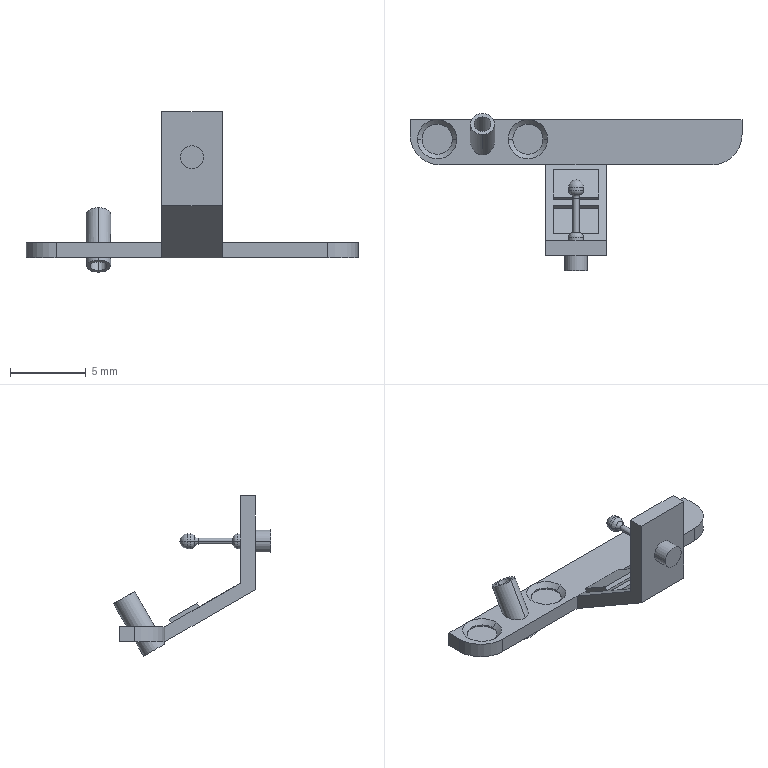Part | SolidWorks | features ICE 5, Revolution 2, Chamfer 1, Extrusion 1, MirrorPattern 1 | 1 solid | 61 faces | box 21.97 x 10.4 x 10.607 mm | volume 112.085 mm3 | plane 29 | cylinder 20 | torus 6 | cone 4 | sphere 2 | commonest cylinder face diameters 1 x4 1.617 x4 2 x4 0.4 x2 1.1 x2 1.5 x2